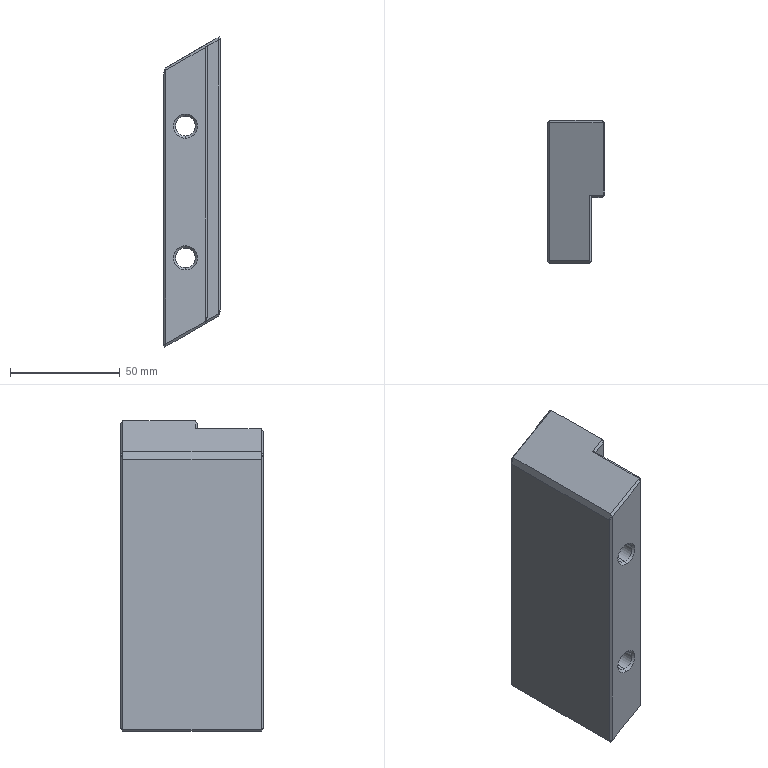Part | STEP file | Trilho - Torre - 1 cav - 1 | 1 solid | 53 faces | box 26 x 65 x 141.296 mm | volume 177227 mm3 | plane 37 | cone 8 | cylinder 8 | commonest cylinder face diameters 9 x4 15 x4